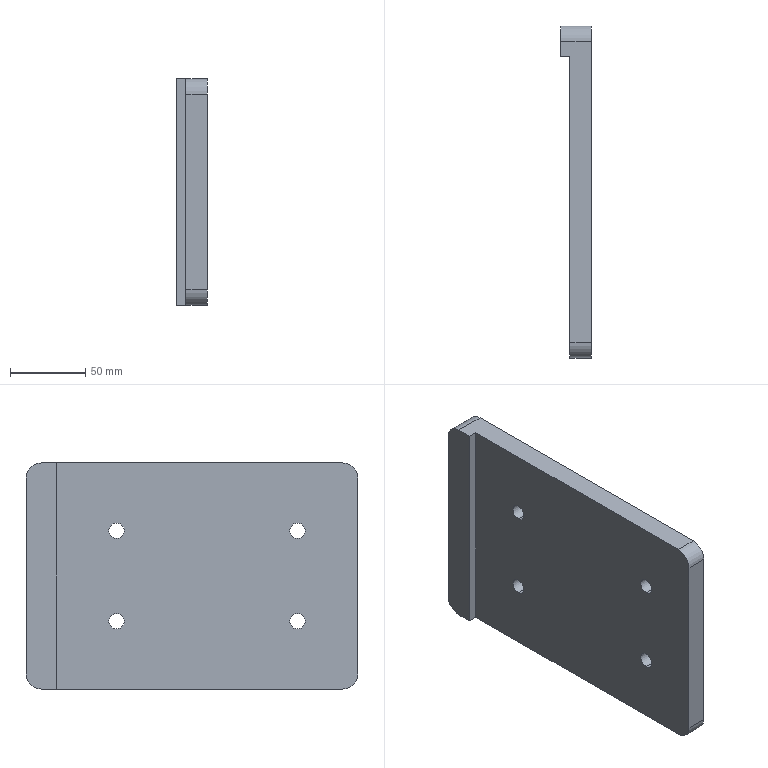Part | SolidWorks | features BaseBody 1 | 1 solid | 20 faces | box 20 x 220 x 150 mm | volume 473965 mm3 | cylinder 12 | plane 8 | commonest cylinder face diameters 10.2 x8 20 x4
STEP:
#1=CARTESIAN_POINT('',(10.,50.,35.1));
#2=VERTEX_POINT('',#1);
#3=CARTESIAN_POINT('',(10.,50.,24.9));
#4=VERTEX_POINT('',#3);
#5=CARTESIAN_POINT('',(10.,50.,30.));
#6=DIRECTION('',(1.,0.,0.));
#7=DIRECTION('',(0.,0.,-1.));
#8=AXIS2_PLACEMENT_3D('',#5,#6,#7);
#9=CIRCLE('',#8,5.1);
#10=EDGE_CURVE('',#2,#4,#9,.T.);
#11=ORIENTED_EDGE('',*,*,#10,.T.);
#12=CARTESIAN_POINT('',(-4.,50.,24.9));
#13=VERTEX_POINT('',#12);
#14=CARTESIAN_POINT('',(-4.,50.,24.9));
#15=DIRECTION('',(-1.,0.,0.));
#16=VECTOR('',#15,1000.);
#17=LINE('',#14,#16);
#18=EDGE_CURVE('',#4,#13,#17,.T.);
#19=ORIENTED_EDGE('',*,*,#18,.T.);
#20=CARTESIAN_POINT('',(-4.,50.,35.1));
#21=VERTEX_POINT('',#20);
#22=CARTESIAN_POINT('',(-4.,50.,30.));
#23=DIRECTION('',(-1.,0.,0.));
#24=DIRECTION('',(0.,0.,1.));
#25=AXIS2_PLACEMENT_3D('',#22,#23,#24);
#26=CIRCLE('',#25,5.1);
#27=EDGE_CURVE('',#13,#21,#26,.T.);
#28=ORIENTED_EDGE('',*,*,#27,.T.);
#29=CARTESIAN_POINT('',(-4.,50.,35.1));
#30=DIRECTION('',(-1.,0.,0.));
#31=VECTOR('',#30,1000.);
#32=LINE('',#29,#31);
#33=EDGE_CURVE('',#2,#21,#32,.T.);
#34=ORIENTED_EDGE('',*,*,#33,.F.);
#35=EDGE_LOOP('',(#11,#19,#28,#34));
#36=FACE_OUTER_BOUND('',#35,.T.);
#37=CARTESIAN_POINT('',(-4.,50.,30.));
#38=DIRECTION('',(-1.,0.,0.));
#39=DIRECTION('',(0.,0.,1.));
#40=AXIS2_PLACEMENT_3D('',#37,#38,#39);
#41=CYLINDRICAL_SURFACE('',#40,5.1);
#42=ADVANCED_FACE('',(#36),#41,.F.);
#43=CARTESIAN_POINT('',(10.,50.,-24.9));
#44=VERTEX_POINT('',#43);
#45=CARTESIAN_POINT('',(10.,50.,-35.1));
#46=VERTEX_POINT('',#45);
#47=CARTESIAN_POINT('',(10.,50.,-30.));
#48=DIRECTION('',(1.,0.,0.));
#49=DIRECTION('',(0.,0.,-1.));
#50=AXIS2_PLACEMENT_3D('',#47,#48,#49);
#51=CIRCLE('',#50,5.1);
#52=EDGE_CURVE('',#44,#46,#51,.T.);
#53=ORIENTED_EDGE('',*,*,#52,.T.);
#54=CARTESIAN_POINT('',(-4.,50.,-35.1));
#55=VERTEX_POINT('',#54);
#56=CARTESIAN_POINT('',(-4.,50.,-35.1));
#57=DIRECTION('',(-1.,0.,0.));
#58=VECTOR('',#57,1000.);
#59=LINE('',#56,#58);
#60=EDGE_CURVE('',#46,#55,#59,.T.);
#61=ORIENTED_EDGE('',*,*,#60,.T.);
#62=CARTESIAN_POINT('',(-4.,50.,-24.9));
#63=VERTEX_POINT('',#62);
#64=CARTESIAN_POINT('',(-4.,50.,-30.));
#65=DIRECTION('',(-1.,0.,0.));
#66=DIRECTION('',(0.,0.,1.));
#67=AXIS2_PLACEMENT_3D('',#64,#65,#66);
#68=CIRCLE('',#67,5.1);
#69=EDGE_CURVE('',#55,#63,#68,.T.);
#70=ORIENTED_EDGE('',*,*,#69,.T.);
#71=CARTESIAN_POINT('',(-4.,50.,-24.9));
#72=DIRECTION('',(-1.,0.,0.));
#73=VECTOR('',#72,1000.);
#74=LINE('',#71,#73);
#75=EDGE_CURVE('',#44,#63,#74,.T.);
#76=ORIENTED_EDGE('',*,*,#75,.F.);
#77=EDGE_LOOP('',(#53,#61,#70,#76));
#78=FACE_OUTER_BOUND('',#77,.T.);
#79=CARTESIAN_POINT('',(-4.,50.,-30.));
#80=DIRECTION('',(-1.,0.,0.));
#81=DIRECTION('',(0.,0.,1.));
#82=AXIS2_PLACEMENT_3D('',#79,#80,#81);
#83=CYLINDRICAL_SURFACE('',#82,5.1);
#84=ADVANCED_FACE('',(#78),#83,.F.);
#85=CARTESIAN_POINT('',(10.,-70.,-24.9));
#86=VERTEX_POINT('',#85);
#87=CARTESIAN_POINT('',(10.,-70.,-35.1));
#88=VERTEX_POINT('',#87);
#89=CARTESIAN_POINT('',(10.,-70.,-30.));
#90=DIRECTION('',(1.,0.,0.));
#91=DIRECTION('',(0.,0.,-1.));
#92=AXIS2_PLACEMENT_3D('',#89,#90,#91);
#93=CIRCLE('',#92,5.1);
#94=EDGE_CURVE('',#86,#88,#93,.T.);
#95=ORIENTED_EDGE('',*,*,#94,.T.);
#96=CARTESIAN_POINT('',(-4.,-70.,-35.1));
#97=VERTEX_POINT('',#96);
#98=CARTESIAN_POINT('',(-4.,-70.,-35.1));
#99=DIRECTION('',(-1.,0.,0.));
#100=VECTOR('',#99,1000.);
#101=LINE('',#98,#100);
#102=EDGE_CURVE('',#88,#97,#101,.T.);
#103=ORIENTED_EDGE('',*,*,#102,.T.);
#104=CARTESIAN_POINT('',(-4.,-70.,-24.9));
#105=VERTEX_POINT('',#104);
#106=CARTESIAN_POINT('',(-4.,-70.,-30.));
#107=DIRECTION('',(-1.,0.,0.));
#108=DIRECTION('',(0.,0.,1.));
#109=AXIS2_PLACEMENT_3D('',#106,#107,#108);
#110=CIRCLE('',#109,5.1);
#111=EDGE_CURVE('',#97,#105,#110,.T.);
#112=ORIENTED_EDGE('',*,*,#111,.T.);
#113=CARTESIAN_POINT('',(-4.,-70.,-24.9));
#114=DIRECTION('',(-1.,0.,0.));
#115=VECTOR('',#114,1000.);
#116=LINE('',#113,#115);
#117=EDGE_CURVE('',#86,#105,#116,.T.);
#118=ORIENTED_EDGE('',*,*,#117,.F.);
#119=EDGE_LOOP('',(#95,#103,#112,#118));
#120=FACE_OUTER_BOUND('',#119,.T.);
#121=CARTESIAN_POINT('',(-4.,-70.,-30.));
#122=DIRECTION('',(-1.,0.,0.));
#123=DIRECTION('',(0.,0.,1.));
#124=AXIS2_PLACEMENT_3D('',#121,#122,#123);
#125=CYLINDRICAL_SURFACE('',#124,5.1);
#126=ADVANCED_FACE('',(#120),#125,.F.);
#127=CARTESIAN_POINT('',(10.,-70.,35.1));
#128=VERTEX_POINT('',#127);
#129=CARTESIAN_POINT('',(10.,-70.,24.9));
#130=VERTEX_POINT('',#129);
#131=CARTESIAN_POINT('',(10.,-70.,30.));
#132=DIRECTION('',(1.,0.,0.));
#133=DIRECTION('',(0.,0.,-1.));
#134=AXIS2_PLACEMENT_3D('',#131,#132,#133);
#135=CIRCLE('',#134,5.1);
#136=EDGE_CURVE('',#128,#130,#135,.T.);
#137=ORIENTED_EDGE('',*,*,#136,.T.);
#138=CARTESIAN_POINT('',(-4.,-70.,24.9));
#139=VERTEX_POINT('',#138);
#140=CARTESIAN_POINT('',(-4.,-70.,24.9));
#141=DIRECTION('',(-1.,0.,0.));
#142=VECTOR('',#141,1000.);
#143=LINE('',#140,#142);
#144=EDGE_CURVE('',#130,#139,#143,.T.);
#145=ORIENTED_EDGE('',*,*,#144,.T.);
#146=CARTESIAN_POINT('',(-4.,-70.,35.1));
#147=VERTEX_POINT('',#146);
#148=CARTESIAN_POINT('',(-4.,-70.,30.));
#149=DIRECTION('',(-1.,0.,0.));
#150=DIRECTION('',(0.,0.,1.));
#151=AXIS2_PLACEMENT_3D('',#148,#149,#150);
#152=CIRCLE('',#151,5.1);
#153=EDGE_CURVE('',#139,#147,#152,.T.);
#154=ORIENTED_EDGE('',*,*,#153,.T.);
#155=CARTESIAN_POINT('',(-4.,-70.,35.1));
#156=DIRECTION('',(-1.,0.,0.));
#157=VECTOR('',#156,1000.);
#158=LINE('',#155,#157);
#159=EDGE_CURVE('',#128,#147,#158,.T.);
#160=ORIENTED_EDGE('',*,*,#159,.F.);
#161=EDGE_LOOP('',(#137,#145,#154,#160));
#162=FACE_OUTER_BOUND('',#161,.T.);
#163=CARTESIAN_POINT('',(-4.,-70.,30.));
#164=DIRECTION('',(-1.,0.,0.));
#165=DIRECTION('',(0.,0.,1.));
#166=AXIS2_PLACEMENT_3D('',#163,#164,#165);
#167=CYLINDRICAL_SURFACE('',#166,5.1);
#168=ADVANCED_FACE('',(#162),#167,.F.);
#169=CARTESIAN_POINT('',(10.,-100.,75.));
#170=VERTEX_POINT('',#169);
#171=CARTESIAN_POINT('',(-4.,-100.,75.));
#172=VERTEX_POINT('',#171);
#173=CARTESIAN_POINT('',(10.,-100.,75.));
#174=DIRECTION('',(-1.,0.,0.));
#175=VECTOR('',#174,1000.);
#176=LINE('',#173,#175);
#177=EDGE_CURVE('',#170,#172,#176,.T.);
#178=ORIENTED_EDGE('',*,*,#177,.T.);
#179=CARTESIAN_POINT('',(-4.,-110.,65.));
#180=VERTEX_POINT('',#179);
#181=CARTESIAN_POINT('',(-4.,-100.,65.));
#182=DIRECTION('',(1.,0.,0.));
#183=DIRECTION('',(0.,0.,-1.));
#184=AXIS2_PLACEMENT_3D('',#181,#182,#183);
#185=CIRCLE('',#184,10.);
#186=EDGE_CURVE('',#172,#180,#185,.T.);
#187=ORIENTED_EDGE('',*,*,#186,.T.);
#188=CARTESIAN_POINT('',(10.,-110.,65.));
#189=VERTEX_POINT('',#188);
#190=CARTESIAN_POINT('',(10.,-110.,65.));
#191=DIRECTION('',(-1.,0.,0.));
#192=VECTOR('',#191,1000.);
#193=LINE('',#190,#192);
#194=EDGE_CURVE('',#189,#180,#193,.T.);
#195=ORIENTED_EDGE('',*,*,#194,.F.);
#196=CARTESIAN_POINT('',(10.,-100.,65.));
#197=DIRECTION('',(1.,0.,0.));
#198=DIRECTION('',(0.,0.,-1.));
#199=AXIS2_PLACEMENT_3D('',#196,#197,#198);
#200=CIRCLE('',#199,10.);
#201=EDGE_CURVE('',#170,#189,#200,.T.);
#202=ORIENTED_EDGE('',*,*,#201,.F.);
#203=EDGE_LOOP('',(#178,#187,#195,#202));
#204=FACE_OUTER_BOUND('',#203,.T.);
#205=CARTESIAN_POINT('',(10.,-100.,65.));
#206=DIRECTION('',(-1.,0.,0.));
#207=DIRECTION('',(0.,0.,1.));
#208=AXIS2_PLACEMENT_3D('',#205,#206,#207);
#209=CYLINDRICAL_SURFACE('',#208,10.);
#210=ADVANCED_FACE('',(#204),#209,.T.);
#211=ORIENTED_EDGE('',*,*,#194,.T.);
#212=CARTESIAN_POINT('',(-4.,-110.,-65.));
#213=VERTEX_POINT('',#212);
#214=CARTESIAN_POINT('',(-4.,-110.,135.));
#215=DIRECTION('',(0.,0.,1.));
#216=VECTOR('',#215,1000.);
#217=LINE('',#214,#216);
#218=EDGE_CURVE('',#213,#180,#217,.T.);
#219=ORIENTED_EDGE('',*,*,#218,.F.);
#220=CARTESIAN_POINT('',(10.,-110.,-65.));
#221=VERTEX_POINT('',#220);
#222=CARTESIAN_POINT('',(10.,-110.,-65.));
#223=DIRECTION('',(-1.,0.,0.));
#224=VECTOR('',#223,1000.);
#225=LINE('',#222,#224);
#226=EDGE_CURVE('',#221,#213,#225,.T.);
#227=ORIENTED_EDGE('',*,*,#226,.F.);
#228=CARTESIAN_POINT('',(10.,-110.,65.));
#229=DIRECTION('',(0.,0.,-1.));
#230=VECTOR('',#229,1000.);
#231=LINE('',#228,#230);
#232=EDGE_CURVE('',#189,#221,#231,.T.);
#233=ORIENTED_EDGE('',*,*,#232,.F.);
#234=EDGE_LOOP('',(#211,#219,#227,#233));
#235=FACE_OUTER_BOUND('',#234,.T.);
#236=CARTESIAN_POINT('',(10.,-110.,65.));
#237=DIRECTION('',(0.,1.,0.));
#238=DIRECTION('',(0.,0.,1.));
#239=AXIS2_PLACEMENT_3D('',#236,#237,#238);
#240=PLANE('',#239);
#241=ADVANCED_FACE('',(#235),#240,.F.);
#242=ORIENTED_EDGE('',*,*,#226,.T.);
#243=CARTESIAN_POINT('',(-4.,-100.,-75.));
#244=VERTEX_POINT('',#243);
#245=CARTESIAN_POINT('',(-4.,-100.,-65.));
#246=DIRECTION('',(1.,0.,0.));
#247=DIRECTION('',(0.,0.,-1.));
#248=AXIS2_PLACEMENT_3D('',#245,#246,#247);
#249=CIRCLE('',#248,10.);
#250=EDGE_CURVE('',#213,#244,#249,.T.);
#251=ORIENTED_EDGE('',*,*,#250,.T.);
#252=CARTESIAN_POINT('',(10.,-100.,-75.));
#253=VERTEX_POINT('',#252);
#254=CARTESIAN_POINT('',(10.,-100.,-75.));
#255=DIRECTION('',(-1.,0.,0.));
#256=VECTOR('',#255,1000.);
#257=LINE('',#254,#256);
#258=EDGE_CURVE('',#253,#244,#257,.T.);
#259=ORIENTED_EDGE('',*,*,#258,.F.);
#260=CARTESIAN_POINT('',(10.,-100.,-65.));
#261=DIRECTION('',(1.,0.,0.));
#262=DIRECTION('',(0.,0.,-1.));
#263=AXIS2_PLACEMENT_3D('',#260,#261,#262);
#264=CIRCLE('',#263,10.);
#265=EDGE_CURVE('',#221,#253,#264,.T.);
#266=ORIENTED_EDGE('',*,*,#265,.F.);
#267=EDGE_LOOP('',(#242,#251,#259,#266));
#268=FACE_OUTER_BOUND('',#267,.T.);
#269=CARTESIAN_POINT('',(10.,-100.,-65.));
#270=DIRECTION('',(-1.,0.,0.));
#271=DIRECTION('',(0.,0.,1.));
#272=AXIS2_PLACEMENT_3D('',#269,#270,#271);
#273=CYLINDRICAL_SURFACE('',#272,10.);
#274=ADVANCED_FACE('',(#268),#273,.T.);
#275=CARTESIAN_POINT('',(-4.,90.,-75.));
#276=VERTEX_POINT('',#275);
#277=CARTESIAN_POINT('',(-4.,90.,-75.));
#278=DIRECTION('',(0.,-1.,0.));
#279=VECTOR('',#278,1000.);
#280=LINE('',#277,#279);
#281=EDGE_CURVE('',#276,#244,#280,.T.);
#282=ORIENTED_EDGE('',*,*,#281,.F.);
#283=CARTESIAN_POINT('',(-10.,90.,-75.));
#284=VERTEX_POINT('',#283);
#285=CARTESIAN_POINT('',(-4.,90.,-75.));
#286=DIRECTION('',(-1.,0.,0.));
#287=VECTOR('',#286,1000.);
#288=LINE('',#285,#287);
#289=EDGE_CURVE('',#276,#284,#288,.T.);
#290=ORIENTED_EDGE('',*,*,#289,.T.);
#291=CARTESIAN_POINT('',(-10.,100.,-75.));
#292=VERTEX_POINT('',#291);
#293=CARTESIAN_POINT('',(-10.,100.,-75.));
#294=DIRECTION('',(0.,1.,0.));
#295=VECTOR('',#294,1000.);
#296=LINE('',#293,#295);
#297=EDGE_CURVE('',#284,#292,#296,.T.);
#298=ORIENTED_EDGE('',*,*,#297,.T.);
#299=CARTESIAN_POINT('',(10.,100.,-75.));
#300=VERTEX_POINT('',#299);
#301=CARTESIAN_POINT('',(10.,100.,-75.));
#302=DIRECTION('',(-1.,0.,0.));
#303=VECTOR('',#302,1000.);
#304=LINE('',#301,#303);
#305=EDGE_CURVE('',#300,#292,#304,.T.);
#306=ORIENTED_EDGE('',*,*,#305,.F.);
#307=CARTESIAN_POINT('',(10.,100.,-75.));
#308=DIRECTION('',(0.,1.,0.));
#309=VECTOR('',#308,1000.);
#310=LINE('',#307,#309);
#311=EDGE_CURVE('',#253,#300,#310,.T.);
#312=ORIENTED_EDGE('',*,*,#311,.F.);
#313=ORIENTED_EDGE('',*,*,#258,.T.);
#314=EDGE_LOOP('',(#282,#290,#298,#306,#312,#313));
#315=FACE_OUTER_BOUND('',#314,.T.);
#316=CARTESIAN_POINT('',(10.,100.,-75.));
#317=DIRECTION('',(0.,0.,1.));
#318=DIRECTION('',(0.,-1.,0.));
#319=AXIS2_PLACEMENT_3D('',#316,#317,#318);
#320=PLANE('',#319);
#321=ADVANCED_FACE('',(#315),#320,.F.);
#322=CARTESIAN_POINT('',(-10.,110.,-65.));
#323=VERTEX_POINT('',#322);
#324=CARTESIAN_POINT('',(-10.,100.,-65.));
#325=DIRECTION('',(1.,0.,0.));
#326=DIRECTION('',(0.,0.,1.));
#327=AXIS2_PLACEMENT_3D('',#324,#325,#326);
#328=CIRCLE('',#327,10.);
#329=EDGE_CURVE('',#292,#323,#328,.T.);
#330=ORIENTED_EDGE('',*,*,#329,.T.);
#331=CARTESIAN_POINT('',(10.,110.,-65.));
#332=VERTEX_POINT('',#331);
#333=CARTESIAN_POINT('',(10.,110.,-65.));
#334=DIRECTION('',(-1.,0.,0.));
#335=VECTOR('',#334,1000.);
#336=LINE('',#333,#335);
#337=EDGE_CURVE('',#332,#323,#336,.T.);
#338=ORIENTED_EDGE('',*,*,#337,.F.);
#339=CARTESIAN_POINT('',(10.,100.,-65.));
#340=DIRECTION('',(1.,0.,0.));
#341=DIRECTION('',(0.,0.,1.));
#342=AXIS2_PLACEMENT_3D('',#339,#340,#341);
#343=CIRCLE('',#342,10.);
#344=EDGE_CURVE('',#300,#332,#343,.T.);
#345=ORIENTED_EDGE('',*,*,#344,.F.);
#346=ORIENTED_EDGE('',*,*,#305,.T.);
#347=EDGE_LOOP('',(#330,#338,#345,#346));
#348=FACE_OUTER_BOUND('',#347,.T.);
#349=CARTESIAN_POINT('',(10.,100.,-65.));
#350=DIRECTION('',(-1.,0.,0.));
#351=DIRECTION('',(0.,0.,1.));
#352=AXIS2_PLACEMENT_3D('',#349,#350,#351);
#353=CYLINDRICAL_SURFACE('',#352,10.);
#354=ADVANCED_FACE('',(#348),#353,.T.);
#355=CARTESIAN_POINT('',(-10.,110.,65.));
#356=VERTEX_POINT('',#355);
#357=CARTESIAN_POINT('',(-10.,110.,65.));
#358=DIRECTION('',(0.,0.,1.));
#359=VECTOR('',#358,1000.);
#360=LINE('',#357,#359);
#361=EDGE_CURVE('',#323,#356,#360,.T.);
#362=ORIENTED_EDGE('',*,*,#361,.T.);
#363=CARTESIAN_POINT('',(10.,110.,65.));
#364=VERTEX_POINT('',#363);
#365=CARTESIAN_POINT('',(10.,110.,65.));
#366=DIRECTION('',(-1.,0.,0.));
#367=VECTOR('',#366,1000.);
#368=LINE('',#365,#367);
#369=EDGE_CURVE('',#364,#356,#368,.T.);
#370=ORIENTED_EDGE('',*,*,#369,.F.);
#371=CARTESIAN_POINT('',(10.,110.,65.));
#372=DIRECTION('',(0.,0.,1.));
#373=VECTOR('',#372,1000.);
#374=LINE('',#371,#373);
#375=EDGE_CURVE('',#332,#364,#374,.T.);
#376=ORIENTED_EDGE('',*,*,#375,.F.);
#377=ORIENTED_EDGE('',*,*,#337,.T.);
#378=EDGE_LOOP('',(#362,#370,#376,#377));
#379=FACE_OUTER_BOUND('',#378,.T.);
#380=CARTESIAN_POINT('',(10.,110.,65.));
#381=DIRECTION('',(0.,-1.,0.));
#382=DIRECTION('',(0.,0.,-1.));
#383=AXIS2_PLACEMENT_3D('',#380,#381,#382);
#384=PLANE('',#383);
#385=ADVANCED_FACE('',(#379),#384,.F.);
#386=CARTESIAN_POINT('',(-10.,100.,75.));
#387=VERTEX_POINT('',#386);
#388=CARTESIAN_POINT('',(-10.,100.,65.));
#389=DIRECTION('',(1.,0.,0.));
#390=DIRECTION('',(0.,0.,-1.));
#391=AXIS2_PLACEMENT_3D('',#388,#389,#390);
#392=CIRCLE('',#391,10.);
#393=EDGE_CURVE('',#356,#387,#392,.T.);
#394=ORIENTED_EDGE('',*,*,#393,.T.);
#395=CARTESIAN_POINT('',(10.,100.,75.));
#396=VERTEX_POINT('',#395);
#397=CARTESIAN_POINT('',(10.,100.,75.));
#398=DIRECTION('',(-1.,0.,0.));
#399=VECTOR('',#398,1000.);
#400=LINE('',#397,#399);
#401=EDGE_CURVE('',#396,#387,#400,.T.);
#402=ORIENTED_EDGE('',*,*,#401,.F.);
#403=CARTESIAN_POINT('',(10.,100.,65.));
#404=DIRECTION('',(1.,0.,0.));
#405=DIRECTION('',(0.,0.,-1.));
#406=AXIS2_PLACEMENT_3D('',#403,#404,#405);
#407=CIRCLE('',#406,10.);
#408=EDGE_CURVE('',#364,#396,#407,.T.);
#409=ORIENTED_EDGE('',*,*,#408,.F.);
#410=ORIENTED_EDGE('',*,*,#369,.T.);
#411=EDGE_LOOP('',(#394,#402,#409,#410));
#412=FACE_OUTER_BOUND('',#411,.T.);
#413=CARTESIAN_POINT('',(10.,100.,65.));
#414=DIRECTION('',(-1.,0.,0.));
#415=DIRECTION('',(0.,0.,1.));
#416=AXIS2_PLACEMENT_3D('',#413,#414,#415);
#417=CYLINDRICAL_SURFACE('',#416,10.);
#418=ADVANCED_FACE('',(#412),#417,.T.);
#419=CARTESIAN_POINT('',(-10.,90.,75.));
#420=VERTEX_POINT('',#419);
#421=CARTESIAN_POINT('',(-10.,100.,75.));
#422=DIRECTION('',(0.,-1.,0.));
#423=VECTOR('',#422,1000.);
#424=LINE('',#421,#423);
#425=EDGE_CURVE('',#387,#420,#424,.T.);
#426=ORIENTED_EDGE('',*,*,#425,.T.);
#427=CARTESIAN_POINT('',(-4.,90.,75.));
#428=VERTEX_POINT('',#427);
#429=CARTESIAN_POINT('',(10.,90.,75.));
#430=DIRECTION('',(1.,0.,0.));
#431=VECTOR('',#430,1000.);
#432=LINE('',#429,#431);
#433=EDGE_CURVE('',#420,#428,#432,.T.);
#434=ORIENTED_EDGE('',*,*,#433,.T.);
#435=CARTESIAN_POINT('',(-4.,100.,75.));
#436=DIRECTION('',(0.,-1.,0.));
#437=VECTOR('',#436,1000.);
#438=LINE('',#435,#437);
#439=EDGE_CURVE('',#428,#172,#438,.T.);
#440=ORIENTED_EDGE('',*,*,#439,.T.);
#441=ORIENTED_EDGE('',*,*,#177,.F.);
#442=CARTESIAN_POINT('',(10.,100.,75.));
#443=DIRECTION('',(0.,-1.,0.));
#444=VECTOR('',#443,1000.);
#445=LINE('',#442,#444);
#446=EDGE_CURVE('',#396,#170,#445,.T.);
#447=ORIENTED_EDGE('',*,*,#446,.F.);
#448=ORIENTED_EDGE('',*,*,#401,.T.);
#449=EDGE_LOOP('',(#426,#434,#440,#441,#447,#448));
#450=FACE_OUTER_BOUND('',#449,.T.);
#451=CARTESIAN_POINT('',(10.,100.,75.));
#452=DIRECTION('',(0.,0.,-1.));
#453=DIRECTION('',(0.,1.,0.));
#454=AXIS2_PLACEMENT_3D('',#451,#452,#453);
#455=PLANE('',#454);
#456=ADVANCED_FACE('',(#450),#455,.F.);
#457=ORIENTED_EDGE('',*,*,#10,.F.);
#458=CARTESIAN_POINT('',(10.,50.,30.));
#459=DIRECTION('',(1.,0.,0.));
#460=DIRECTION('',(0.,0.,-1.));
#461=AXIS2_PLACEMENT_3D('',#458,#459,#460);
#462=CIRCLE('',#461,5.1);
#463=EDGE_CURVE('',#4,#2,#462,.T.);
#464=ORIENTED_EDGE('',*,*,#463,.F.);
#465=EDGE_LOOP('',(#457,#464));
#466=FACE_BOUND('',#465,.T.);
#467=ORIENTED_EDGE('',*,*,#52,.F.);
#468=CARTESIAN_POINT('',(10.,50.,-30.));
#469=DIRECTION('',(1.,0.,0.));
#470=DIRECTION('',(0.,0.,-1.));
#471=AXIS2_PLACEMENT_3D('',#468,#469,#470);
#472=CIRCLE('',#471,5.1);
#473=EDGE_CURVE('',#46,#44,#472,.T.);
#474=ORIENTED_EDGE('',*,*,#473,.F.);
#475=EDGE_LOOP('',(#467,#474));
#476=FACE_BOUND('',#475,.T.);
#477=ORIENTED_EDGE('',*,*,#94,.F.);
#478=CARTESIAN_POINT('',(10.,-70.,-30.));
#479=DIRECTION('',(1.,0.,0.));
#480=DIRECTION('',(0.,0.,-1.));
#481=AXIS2_PLACEMENT_3D('',#478,#479,#480);
#482=CIRCLE('',#481,5.1);
#483=EDGE_CURVE('',#88,#86,#482,.T.);
#484=ORIENTED_EDGE('',*,*,#483,.F.);
#485=EDGE_LOOP('',(#477,#484));
#486=FACE_BOUND('',#485,.T.);
#487=ORIENTED_EDGE('',*,*,#136,.F.);
#488=CARTESIAN_POINT('',(10.,-70.,30.));
#489=DIRECTION('',(1.,0.,0.));
#490=DIRECTION('',(0.,0.,-1.));
#491=AXIS2_PLACEMENT_3D('',#488,#489,#490);
#492=CIRCLE('',#491,5.1);
#493=EDGE_CURVE('',#130,#128,#492,.T.);
#494=ORIENTED_EDGE('',*,*,#493,.F.);
#495=EDGE_LOOP('',(#487,#494));
#496=FACE_BOUND('',#495,.T.);
#497=ORIENTED_EDGE('',*,*,#201,.T.);
#498=ORIENTED_EDGE('',*,*,#232,.T.);
#499=ORIENTED_EDGE('',*,*,#265,.T.);
#500=ORIENTED_EDGE('',*,*,#311,.T.);
#501=ORIENTED_EDGE('',*,*,#344,.T.);
#502=ORIENTED_EDGE('',*,*,#375,.T.);
#503=ORIENTED_EDGE('',*,*,#408,.T.);
#504=ORIENTED_EDGE('',*,*,#446,.T.);
#505=EDGE_LOOP('',(#497,#498,#499,#500,#501,#502,#503,#504));
#506=FACE_OUTER_BOUND('',#505,.T.);
#507=CARTESIAN_POINT('',(10.,-100.,65.));
#508=DIRECTION('',(1.,0.,0.));
#509=DIRECTION('',(0.,0.,-1.));
#510=AXIS2_PLACEMENT_3D('',#507,#508,#509);
#511=PLANE('',#510);
#512=ADVANCED_FACE('',(#466,#476,#486,#496,#506),#511,.T.);
#513=ORIENTED_EDGE('',*,*,#297,.F.);
#514=CARTESIAN_POINT('',(-10.,90.,65.));
#515=DIRECTION('',(0.,0.,1.));
#516=VECTOR('',#515,1000.);
#517=LINE('',#514,#516);
#518=EDGE_CURVE('',#284,#420,#517,.T.);
#519=ORIENTED_EDGE('',*,*,#518,.T.);
#520=ORIENTED_EDGE('',*,*,#425,.F.);
#521=ORIENTED_EDGE('',*,*,#393,.F.);
#522=ORIENTED_EDGE('',*,*,#361,.F.);
#523=ORIENTED_EDGE('',*,*,#329,.F.);
#524=EDGE_LOOP('',(#513,#519,#520,#521,#522,#523));
#525=FACE_OUTER_BOUND('',#524,.T.);
#526=CARTESIAN_POINT('',(-10.,-100.,65.));
#527=DIRECTION('',(1.,0.,0.));
#528=DIRECTION('',(0.,0.,-1.));
#529=AXIS2_PLACEMENT_3D('',#526,#527,#528);
#530=PLANE('',#529);
#531=ADVANCED_FACE('',(#525),#530,.F.);
#532=CARTESIAN_POINT('',(-4.,50.,30.));
#533=DIRECTION('',(-1.,0.,0.));
#534=DIRECTION('',(0.,0.,1.));
#535=AXIS2_PLACEMENT_3D('',#532,#533,#534);
#536=CIRCLE('',#535,5.1);
#537=EDGE_CURVE('',#21,#13,#536,.T.);
#538=ORIENTED_EDGE('',*,*,#537,.F.);
#539=ORIENTED_EDGE('',*,*,#27,.F.);
#540=EDGE_LOOP('',(#538,#539));
#541=FACE_BOUND('',#540,.T.);
#542=CARTESIAN_POINT('',(-4.,50.,-30.));
#543=DIRECTION('',(-1.,0.,0.));
#544=DIRECTION('',(0.,0.,1.));
#545=AXIS2_PLACEMENT_3D('',#542,#543,#544);
#546=CIRCLE('',#545,5.1);
#547=EDGE_CURVE('',#63,#55,#546,.T.);
#548=ORIENTED_EDGE('',*,*,#547,.F.);
#549=ORIENTED_EDGE('',*,*,#69,.F.);
#550=EDGE_LOOP('',(#548,#549));
#551=FACE_BOUND('',#550,.T.);
#552=CARTESIAN_POINT('',(-4.,-70.,-30.));
#553=DIRECTION('',(-1.,0.,0.));
#554=DIRECTION('',(0.,0.,1.));
#555=AXIS2_PLACEMENT_3D('',#552,#553,#554);
#556=CIRCLE('',#555,5.1);
#557=EDGE_CURVE('',#105,#97,#556,.T.);
#558=ORIENTED_EDGE('',*,*,#557,.F.);
#559=ORIENTED_EDGE('',*,*,#111,.F.);
#560=EDGE_LOOP('',(#558,#559));
#561=FACE_BOUND('',#560,.T.);
#562=CARTESIAN_POINT('',(-4.,-70.,30.));
#563=DIRECTION('',(-1.,0.,0.));
#564=DIRECTION('',(0.,0.,1.));
#565=AXIS2_PLACEMENT_3D('',#562,#563,#564);
#566=CIRCLE('',#565,5.1);
#567=EDGE_CURVE('',#147,#139,#566,.T.);
#568=ORIENTED_EDGE('',*,*,#567,.F.);
#569=ORIENTED_EDGE('',*,*,#153,.F.);
#570=EDGE_LOOP('',(#568,#569));
#571=FACE_BOUND('',#570,.T.);
#572=ORIENTED_EDGE('',*,*,#218,.T.);
#573=ORIENTED_EDGE('',*,*,#186,.F.);
#574=ORIENTED_EDGE('',*,*,#439,.F.);
#575=CARTESIAN_POINT('',(-4.,90.,135.));
#576=DIRECTION('',(0.,0.,-1.));
#577=VECTOR('',#576,1000.);
#578=LINE('',#575,#577);
#579=EDGE_CURVE('',#428,#276,#578,.T.);
#580=ORIENTED_EDGE('',*,*,#579,.T.);
#581=ORIENTED_EDGE('',*,*,#281,.T.);
#582=ORIENTED_EDGE('',*,*,#250,.F.);
#583=EDGE_LOOP('',(#572,#573,#574,#580,#581,#582));
#584=FACE_OUTER_BOUND('',#583,.T.);
#585=CARTESIAN_POINT('',(-4.,190.64,-577.5));
#586=DIRECTION('',(1.,0.,0.));
#587=DIRECTION('',(0.,0.,-1.));
#588=AXIS2_PLACEMENT_3D('',#585,#586,#587);
#589=PLANE('',#588);
#590=ADVANCED_FACE('',(#541,#551,#561,#571,#584),#589,.F.);
#591=ORIENTED_EDGE('',*,*,#518,.F.);
#592=ORIENTED_EDGE('',*,*,#289,.F.);
#593=ORIENTED_EDGE('',*,*,#579,.F.);
#594=ORIENTED_EDGE('',*,*,#433,.F.);
#595=EDGE_LOOP('',(#591,#592,#593,#594));
#596=FACE_OUTER_BOUND('',#595,.T.);
#597=CARTESIAN_POINT('',(-4.,90.,135.));
#598=DIRECTION('',(0.,1.,0.));
#599=DIRECTION('',(0.,0.,1.));
#600=AXIS2_PLACEMENT_3D('',#597,#598,#599);
#601=PLANE('',#600);
#602=ADVANCED_FACE('',(#596),#601,.F.);
#603=ORIENTED_EDGE('',*,*,#144,.F.);
#604=ORIENTED_EDGE('',*,*,#493,.T.);
#605=ORIENTED_EDGE('',*,*,#159,.T.);
#606=ORIENTED_EDGE('',*,*,#567,.T.);
#607=EDGE_LOOP('',(#603,#604,#605,#606));
#608=FACE_OUTER_BOUND('',#607,.T.);
#609=CARTESIAN_POINT('',(-4.,-70.,30.));
#610=DIRECTION('',(-1.,0.,0.));
#611=DIRECTION('',(0.,0.,1.));
#612=AXIS2_PLACEMENT_3D('',#609,#610,#611);
#613=CYLINDRICAL_SURFACE('',#612,5.1);
#614=ADVANCED_FACE('',(#608),#613,.F.);
#615=ORIENTED_EDGE('',*,*,#102,.F.);
#616=ORIENTED_EDGE('',*,*,#483,.T.);
#617=ORIENTED_EDGE('',*,*,#117,.T.);
#618=ORIENTED_EDGE('',*,*,#557,.T.);
#619=EDGE_LOOP('',(#615,#616,#617,#618));
#620=FACE_OUTER_BOUND('',#619,.T.);
#621=CARTESIAN_POINT('',(-4.,-70.,-30.));
#622=DIRECTION('',(-1.,0.,0.));
#623=DIRECTION('',(0.,0.,1.));
#624=AXIS2_PLACEMENT_3D('',#621,#622,#623);
#625=CYLINDRICAL_SURFACE('',#624,5.1);
#626=ADVANCED_FACE('',(#620),#625,.F.);
#627=ORIENTED_EDGE('',*,*,#60,.F.);
#628=ORIENTED_EDGE('',*,*,#473,.T.);
#629=ORIENTED_EDGE('',*,*,#75,.T.);
#630=ORIENTED_EDGE('',*,*,#547,.T.);
#631=EDGE_LOOP('',(#627,#628,#629,#630));
#632=FACE_OUTER_BOUND('',#631,.T.);
#633=CARTESIAN_POINT('',(-4.,50.,-30.));
#634=DIRECTION('',(-1.,0.,0.));
#635=DIRECTION('',(0.,0.,1.));
#636=AXIS2_PLACEMENT_3D('',#633,#634,#635);
#637=CYLINDRICAL_SURFACE('',#636,5.1);
#638=ADVANCED_FACE('',(#632),#637,.F.);
#639=ORIENTED_EDGE('',*,*,#18,.F.);
#640=ORIENTED_EDGE('',*,*,#463,.T.);
#641=ORIENTED_EDGE('',*,*,#33,.T.);
#642=ORIENTED_EDGE('',*,*,#537,.T.);
#643=EDGE_LOOP('',(#639,#640,#641,#642));
#644=FACE_OUTER_BOUND('',#643,.T.);
#645=CARTESIAN_POINT('',(-4.,50.,30.));
#646=DIRECTION('',(-1.,0.,0.));
#647=DIRECTION('',(0.,0.,1.));
#648=AXIS2_PLACEMENT_3D('',#645,#646,#647);
#649=CYLINDRICAL_SURFACE('',#648,5.1);
#650=ADVANCED_FACE('',(#644),#649,.F.);
#651=CLOSED_SHELL('',(#42,#84,#126,#168,#210,#241,#274,#321,#354,#385,#418,#456,#512,#531,#590,#602,#614,#626,#638,#650));
#652=MANIFOLD_SOLID_BREP('',#651);
#653=CARTESIAN_POINT('',(0.,0.,0.));
#654=DIRECTION('',(0.,0.,1.));
#655=DIRECTION('',(1.,0.,0.));
#656=AXIS2_PLACEMENT_3D('',#653,#654,#655);
#657=(LENGTH_UNIT()NAMED_UNIT(*)SI_UNIT(.MILLI.,.METRE.));
#658=UNCERTAINTY_MEASURE_WITH_UNIT(LENGTH_MEASURE(0.00001),#657,'','');
#659=(NAMED_UNIT(*)PLANE_ANGLE_UNIT()SI_UNIT($,.RADIAN.));
#660=(NAMED_UNIT(*)SI_UNIT($,.STERADIAN.)SOLID_ANGLE_UNIT());
#661=(GEOMETRIC_REPRESENTATION_CONTEXT(3)GLOBAL_UNCERTAINTY_ASSIGNED_CONTEXT((#658))GLOBAL_UNIT_ASSIGNED_CONTEXT((#657,#659,#660))REPRESENTATION_CONTEXT('',''));
#662=ADVANCED_BREP_SHAPE_REPRESENTATION('',(#652,#656),#661);